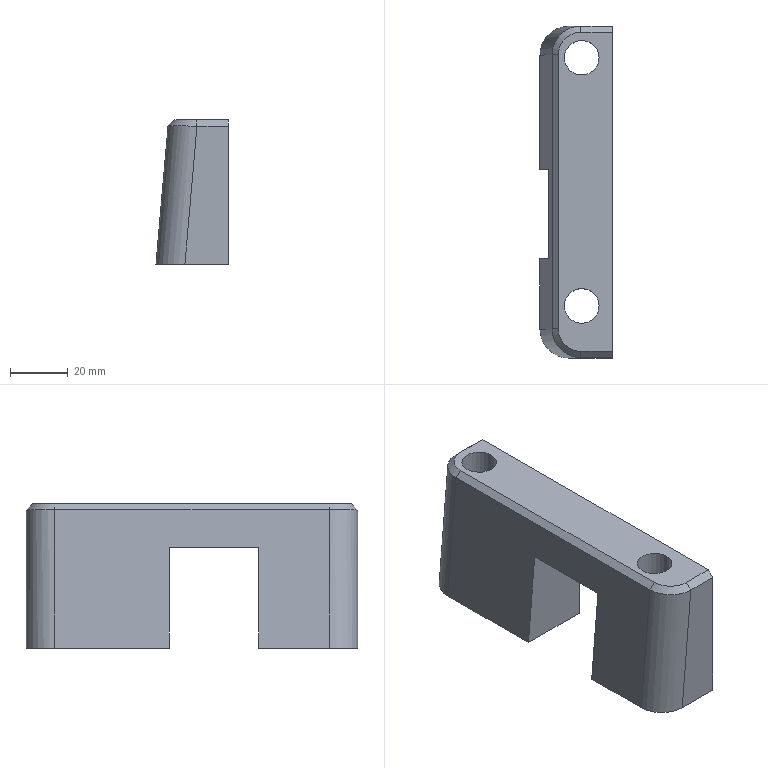Part | STEP file | solid 74 | 1 solid | 23 faces | box 25 x 115 x 50 mm | volume 88592 mm3 | plane 15 | cylinder 6 | spline 2 | commonest cylinder face diameters 12 x2 18 x2 20 x2